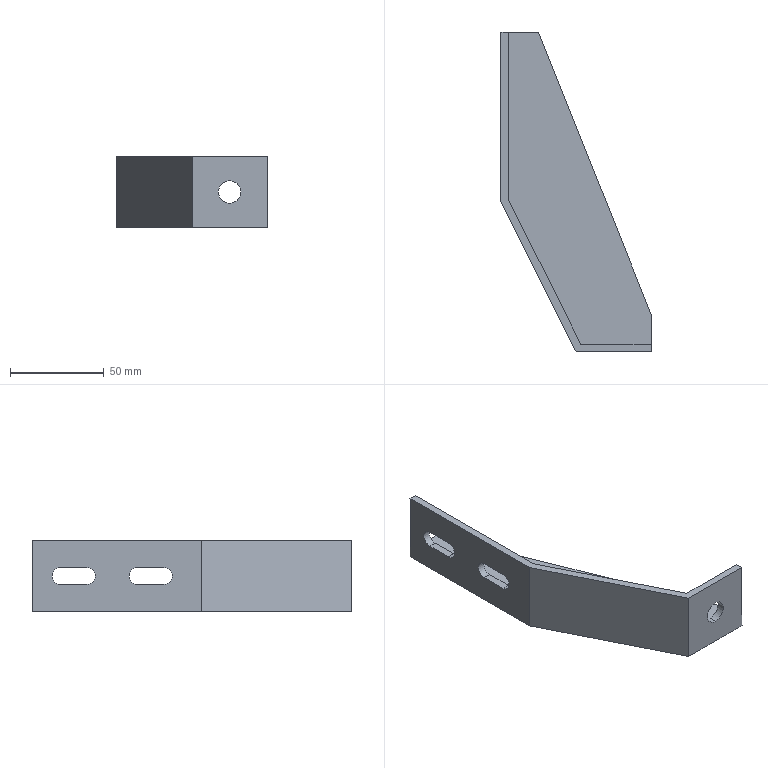Part | STEP file | 1 solid | 24 faces | box 80 x 170 x 38 mm | volume 57410 mm3 | plane 16 | cylinder 8 | commonest cylinder face diameters 9 x6 12 x2